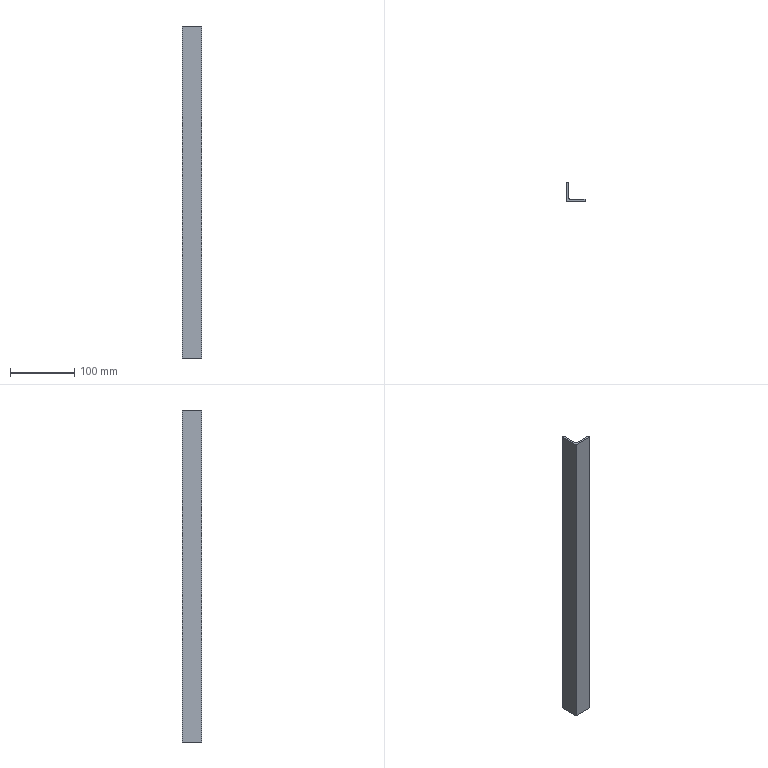Part | SolidWorks | features Extrusion 1 | 1 solid | 11 faces | box 30 x 30 x 515 mm | volume 90082 mm3 | plane 8 | cylinder 3 | commonest cylinder face diameters 2 x2 9 x1
STEP:
#1=CARTESIAN_POINT('',(2.,30.,-257.5));
#2=VERTEX_POINT('',#1);
#3=CARTESIAN_POINT('',(3.,29.,-257.5));
#4=VERTEX_POINT('',#3);
#5=CARTESIAN_POINT('',(2.,29.,-257.5));
#6=DIRECTION('',(0.,0.,-1.));
#7=DIRECTION('',(-1.,0.,0.));
#8=AXIS2_PLACEMENT_3D('',#5,#6,#7);
#9=CIRCLE('',#8,1.);
#10=EDGE_CURVE('',#2,#4,#9,.T.);
#11=ORIENTED_EDGE('',*,*,#10,.F.);
#12=CARTESIAN_POINT('',(2.,30.,257.5));
#13=VERTEX_POINT('',#12);
#14=CARTESIAN_POINT('',(2.,30.,257.5));
#15=DIRECTION('',(0.,0.,-1.));
#16=VECTOR('',#15,1000.);
#17=LINE('',#14,#16);
#18=EDGE_CURVE('',#13,#2,#17,.T.);
#19=ORIENTED_EDGE('',*,*,#18,.F.);
#20=CARTESIAN_POINT('',(3.,29.,257.5));
#21=VERTEX_POINT('',#20);
#22=CARTESIAN_POINT('',(2.,29.,257.5));
#23=DIRECTION('',(0.,0.,-1.));
#24=DIRECTION('',(-1.,0.,0.));
#25=AXIS2_PLACEMENT_3D('',#22,#23,#24);
#26=CIRCLE('',#25,1.);
#27=EDGE_CURVE('',#13,#21,#26,.T.);
#28=ORIENTED_EDGE('',*,*,#27,.T.);
#29=CARTESIAN_POINT('',(3.,29.,257.5));
#30=DIRECTION('',(0.,0.,-1.));
#31=VECTOR('',#30,1000.);
#32=LINE('',#29,#31);
#33=EDGE_CURVE('',#21,#4,#32,.T.);
#34=ORIENTED_EDGE('',*,*,#33,.T.);
#35=EDGE_LOOP('',(#11,#19,#28,#34));
#36=FACE_OUTER_BOUND('',#35,.T.);
#37=CARTESIAN_POINT('',(2.,29.,257.5));
#38=DIRECTION('',(0.,0.,-1.));
#39=DIRECTION('',(-1.,0.,0.));
#40=AXIS2_PLACEMENT_3D('',#37,#38,#39);
#41=CYLINDRICAL_SURFACE('',#40,1.);
#42=ADVANCED_FACE('',(#36),#41,.T.);
#43=CARTESIAN_POINT('',(0.,30.,-257.5));
#44=VERTEX_POINT('',#43);
#45=CARTESIAN_POINT('',(0.,30.,-257.5));
#46=DIRECTION('',(1.,0.,0.));
#47=VECTOR('',#46,1000.);
#48=LINE('',#45,#47);
#49=EDGE_CURVE('',#44,#2,#48,.T.);
#50=ORIENTED_EDGE('',*,*,#49,.F.);
#51=CARTESIAN_POINT('',(0.,30.,257.5));
#52=VERTEX_POINT('',#51);
#53=CARTESIAN_POINT('',(0.,30.,257.5));
#54=DIRECTION('',(0.,0.,-1.));
#55=VECTOR('',#54,1000.);
#56=LINE('',#53,#55);
#57=EDGE_CURVE('',#52,#44,#56,.T.);
#58=ORIENTED_EDGE('',*,*,#57,.F.);
#59=CARTESIAN_POINT('',(0.,30.,257.5));
#60=DIRECTION('',(1.,0.,0.));
#61=VECTOR('',#60,1000.);
#62=LINE('',#59,#61);
#63=EDGE_CURVE('',#52,#13,#62,.T.);
#64=ORIENTED_EDGE('',*,*,#63,.T.);
#65=ORIENTED_EDGE('',*,*,#18,.T.);
#66=EDGE_LOOP('',(#50,#58,#64,#65));
#67=FACE_OUTER_BOUND('',#66,.T.);
#68=CARTESIAN_POINT('',(0.,30.,257.5));
#69=DIRECTION('',(0.,1.,0.));
#70=DIRECTION('',(0.,0.,1.));
#71=AXIS2_PLACEMENT_3D('',#68,#69,#70);
#72=PLANE('',#71);
#73=ADVANCED_FACE('',(#67),#72,.T.);
#74=CARTESIAN_POINT('',(0.,0.,-257.5));
#75=VERTEX_POINT('',#74);
#76=CARTESIAN_POINT('',(0.,0.,-257.5));
#77=DIRECTION('',(0.,1.,0.));
#78=VECTOR('',#77,1000.);
#79=LINE('',#76,#78);
#80=EDGE_CURVE('',#75,#44,#79,.T.);
#81=ORIENTED_EDGE('',*,*,#80,.F.);
#82=CARTESIAN_POINT('',(0.,0.,257.5));
#83=VERTEX_POINT('',#82);
#84=CARTESIAN_POINT('',(0.,0.,257.5));
#85=DIRECTION('',(0.,0.,-1.));
#86=VECTOR('',#85,1000.);
#87=LINE('',#84,#86);
#88=EDGE_CURVE('',#83,#75,#87,.T.);
#89=ORIENTED_EDGE('',*,*,#88,.F.);
#90=CARTESIAN_POINT('',(0.,0.,257.5));
#91=DIRECTION('',(0.,1.,0.));
#92=VECTOR('',#91,1000.);
#93=LINE('',#90,#92);
#94=EDGE_CURVE('',#83,#52,#93,.T.);
#95=ORIENTED_EDGE('',*,*,#94,.T.);
#96=ORIENTED_EDGE('',*,*,#57,.T.);
#97=EDGE_LOOP('',(#81,#89,#95,#96));
#98=FACE_OUTER_BOUND('',#97,.T.);
#99=CARTESIAN_POINT('',(0.,0.,257.5));
#100=DIRECTION('',(-1.,0.,0.));
#101=DIRECTION('',(0.,0.,1.));
#102=AXIS2_PLACEMENT_3D('',#99,#100,#101);
#103=PLANE('',#102);
#104=ADVANCED_FACE('',(#98),#103,.T.);
#105=CARTESIAN_POINT('',(30.,0.,-257.5));
#106=VERTEX_POINT('',#105);
#107=CARTESIAN_POINT('',(30.,0.,-257.5));
#108=DIRECTION('',(-1.,0.,0.));
#109=VECTOR('',#108,1000.);
#110=LINE('',#107,#109);
#111=EDGE_CURVE('',#106,#75,#110,.T.);
#112=ORIENTED_EDGE('',*,*,#111,.F.);
#113=CARTESIAN_POINT('',(30.,0.,257.5));
#114=VERTEX_POINT('',#113);
#115=CARTESIAN_POINT('',(30.,0.,257.5));
#116=DIRECTION('',(0.,0.,-1.));
#117=VECTOR('',#116,1000.);
#118=LINE('',#115,#117);
#119=EDGE_CURVE('',#114,#106,#118,.T.);
#120=ORIENTED_EDGE('',*,*,#119,.F.);
#121=CARTESIAN_POINT('',(30.,0.,257.5));
#122=DIRECTION('',(-1.,0.,0.));
#123=VECTOR('',#122,1000.);
#124=LINE('',#121,#123);
#125=EDGE_CURVE('',#114,#83,#124,.T.);
#126=ORIENTED_EDGE('',*,*,#125,.T.);
#127=ORIENTED_EDGE('',*,*,#88,.T.);
#128=EDGE_LOOP('',(#112,#120,#126,#127));
#129=FACE_OUTER_BOUND('',#128,.T.);
#130=CARTESIAN_POINT('',(30.,0.,257.5));
#131=DIRECTION('',(0.,-1.,0.));
#132=DIRECTION('',(0.,0.,-1.));
#133=AXIS2_PLACEMENT_3D('',#130,#131,#132);
#134=PLANE('',#133);
#135=ADVANCED_FACE('',(#129),#134,.T.);
#136=CARTESIAN_POINT('',(30.,2.,-257.5));
#137=VERTEX_POINT('',#136);
#138=CARTESIAN_POINT('',(30.,0.,-257.5));
#139=DIRECTION('',(0.,1.,0.));
#140=VECTOR('',#139,1000.);
#141=LINE('',#138,#140);
#142=EDGE_CURVE('',#106,#137,#141,.T.);
#143=ORIENTED_EDGE('',*,*,#142,.T.);
#144=CARTESIAN_POINT('',(30.,2.,257.5));
#145=VERTEX_POINT('',#144);
#146=CARTESIAN_POINT('',(30.,2.,257.5));
#147=DIRECTION('',(0.,0.,-1.));
#148=VECTOR('',#147,1000.);
#149=LINE('',#146,#148);
#150=EDGE_CURVE('',#145,#137,#149,.T.);
#151=ORIENTED_EDGE('',*,*,#150,.F.);
#152=CARTESIAN_POINT('',(30.,0.,257.5));
#153=DIRECTION('',(0.,1.,0.));
#154=VECTOR('',#153,1000.);
#155=LINE('',#152,#154);
#156=EDGE_CURVE('',#114,#145,#155,.T.);
#157=ORIENTED_EDGE('',*,*,#156,.F.);
#158=ORIENTED_EDGE('',*,*,#119,.T.);
#159=EDGE_LOOP('',(#143,#151,#157,#158));
#160=FACE_OUTER_BOUND('',#159,.T.);
#161=CARTESIAN_POINT('',(30.,0.,257.5));
#162=DIRECTION('',(-1.,0.,0.));
#163=DIRECTION('',(0.,0.,1.));
#164=AXIS2_PLACEMENT_3D('',#161,#162,#163);
#165=PLANE('',#164);
#166=ADVANCED_FACE('',(#160),#165,.F.);
#167=CARTESIAN_POINT('',(29.,3.,-257.5));
#168=VERTEX_POINT('',#167);
#169=CARTESIAN_POINT('',(29.,2.,-257.5));
#170=DIRECTION('',(0.,0.,1.));
#171=DIRECTION('',(1.,0.,0.));
#172=AXIS2_PLACEMENT_3D('',#169,#170,#171);
#173=CIRCLE('',#172,1.);
#174=EDGE_CURVE('',#137,#168,#173,.T.);
#175=ORIENTED_EDGE('',*,*,#174,.T.);
#176=CARTESIAN_POINT('',(29.,3.,257.5));
#177=VERTEX_POINT('',#176);
#178=CARTESIAN_POINT('',(29.,3.,257.5));
#179=DIRECTION('',(0.,0.,-1.));
#180=VECTOR('',#179,1000.);
#181=LINE('',#178,#180);
#182=EDGE_CURVE('',#177,#168,#181,.T.);
#183=ORIENTED_EDGE('',*,*,#182,.F.);
#184=CARTESIAN_POINT('',(29.,2.,257.5));
#185=DIRECTION('',(0.,0.,1.));
#186=DIRECTION('',(1.,0.,0.));
#187=AXIS2_PLACEMENT_3D('',#184,#185,#186);
#188=CIRCLE('',#187,1.);
#189=EDGE_CURVE('',#145,#177,#188,.T.);
#190=ORIENTED_EDGE('',*,*,#189,.F.);
#191=ORIENTED_EDGE('',*,*,#150,.T.);
#192=EDGE_LOOP('',(#175,#183,#190,#191));
#193=FACE_OUTER_BOUND('',#192,.T.);
#194=CARTESIAN_POINT('',(29.,2.,257.5));
#195=DIRECTION('',(0.,0.,-1.));
#196=DIRECTION('',(-1.,0.,0.));
#197=AXIS2_PLACEMENT_3D('',#194,#195,#196);
#198=CYLINDRICAL_SURFACE('',#197,1.);
#199=ADVANCED_FACE('',(#193),#198,.T.);
#200=CARTESIAN_POINT('',(7.5,3.,-257.5));
#201=VERTEX_POINT('',#200);
#202=CARTESIAN_POINT('',(7.5,3.,-257.5));
#203=DIRECTION('',(1.,0.,0.));
#204=VECTOR('',#203,1000.);
#205=LINE('',#202,#204);
#206=EDGE_CURVE('',#201,#168,#205,.T.);
#207=ORIENTED_EDGE('',*,*,#206,.F.);
#208=CARTESIAN_POINT('',(7.5,3.,257.5));
#209=VERTEX_POINT('',#208);
#210=CARTESIAN_POINT('',(7.5,3.,257.5));
#211=DIRECTION('',(0.,0.,-1.));
#212=VECTOR('',#211,1000.);
#213=LINE('',#210,#212);
#214=EDGE_CURVE('',#209,#201,#213,.T.);
#215=ORIENTED_EDGE('',*,*,#214,.F.);
#216=CARTESIAN_POINT('',(7.5,3.,257.5));
#217=DIRECTION('',(1.,0.,0.));
#218=VECTOR('',#217,1000.);
#219=LINE('',#216,#218);
#220=EDGE_CURVE('',#209,#177,#219,.T.);
#221=ORIENTED_EDGE('',*,*,#220,.T.);
#222=ORIENTED_EDGE('',*,*,#182,.T.);
#223=EDGE_LOOP('',(#207,#215,#221,#222));
#224=FACE_OUTER_BOUND('',#223,.T.);
#225=CARTESIAN_POINT('',(7.5,3.,257.5));
#226=DIRECTION('',(0.,1.,0.));
#227=DIRECTION('',(-1.,0.,0.));
#228=AXIS2_PLACEMENT_3D('',#225,#226,#227);
#229=PLANE('',#228);
#230=ADVANCED_FACE('',(#224),#229,.T.);
#231=CARTESIAN_POINT('',(3.,7.5,-257.5));
#232=VERTEX_POINT('',#231);
#233=CARTESIAN_POINT('',(7.5,7.5,-257.5));
#234=DIRECTION('',(0.,0.,-1.));
#235=DIRECTION('',(-1.,0.,0.));
#236=AXIS2_PLACEMENT_3D('',#233,#234,#235);
#237=CIRCLE('',#236,4.5);
#238=EDGE_CURVE('',#201,#232,#237,.T.);
#239=ORIENTED_EDGE('',*,*,#238,.T.);
#240=CARTESIAN_POINT('',(3.,7.5,257.5));
#241=VERTEX_POINT('',#240);
#242=CARTESIAN_POINT('',(3.,7.5,257.5));
#243=DIRECTION('',(0.,0.,-1.));
#244=VECTOR('',#243,1000.);
#245=LINE('',#242,#244);
#246=EDGE_CURVE('',#241,#232,#245,.T.);
#247=ORIENTED_EDGE('',*,*,#246,.F.);
#248=CARTESIAN_POINT('',(7.5,7.5,257.5));
#249=DIRECTION('',(0.,0.,-1.));
#250=DIRECTION('',(-1.,0.,0.));
#251=AXIS2_PLACEMENT_3D('',#248,#249,#250);
#252=CIRCLE('',#251,4.5);
#253=EDGE_CURVE('',#209,#241,#252,.T.);
#254=ORIENTED_EDGE('',*,*,#253,.F.);
#255=ORIENTED_EDGE('',*,*,#214,.T.);
#256=EDGE_LOOP('',(#239,#247,#254,#255));
#257=FACE_OUTER_BOUND('',#256,.T.);
#258=CARTESIAN_POINT('',(7.5,7.5,257.5));
#259=DIRECTION('',(0.,0.,-1.));
#260=DIRECTION('',(-1.,0.,0.));
#261=AXIS2_PLACEMENT_3D('',#258,#259,#260);
#262=CYLINDRICAL_SURFACE('',#261,4.5);
#263=ADVANCED_FACE('',(#257),#262,.F.);
#264=CARTESIAN_POINT('',(3.,29.,-257.5));
#265=DIRECTION('',(0.,-1.,0.));
#266=VECTOR('',#265,1000.);
#267=LINE('',#264,#266);
#268=EDGE_CURVE('',#4,#232,#267,.T.);
#269=ORIENTED_EDGE('',*,*,#268,.F.);
#270=ORIENTED_EDGE('',*,*,#33,.F.);
#271=CARTESIAN_POINT('',(3.,29.,257.5));
#272=DIRECTION('',(0.,-1.,0.));
#273=VECTOR('',#272,1000.);
#274=LINE('',#271,#273);
#275=EDGE_CURVE('',#21,#241,#274,.T.);
#276=ORIENTED_EDGE('',*,*,#275,.T.);
#277=ORIENTED_EDGE('',*,*,#246,.T.);
#278=EDGE_LOOP('',(#269,#270,#276,#277));
#279=FACE_OUTER_BOUND('',#278,.T.);
#280=CARTESIAN_POINT('',(3.,29.,257.5));
#281=DIRECTION('',(1.,0.,0.));
#282=DIRECTION('',(0.,1.,0.));
#283=AXIS2_PLACEMENT_3D('',#280,#281,#282);
#284=PLANE('',#283);
#285=ADVANCED_FACE('',(#279),#284,.T.);
#286=ORIENTED_EDGE('',*,*,#27,.F.);
#287=ORIENTED_EDGE('',*,*,#63,.F.);
#288=ORIENTED_EDGE('',*,*,#94,.F.);
#289=ORIENTED_EDGE('',*,*,#125,.F.);
#290=ORIENTED_EDGE('',*,*,#156,.T.);
#291=ORIENTED_EDGE('',*,*,#189,.T.);
#292=ORIENTED_EDGE('',*,*,#220,.F.);
#293=ORIENTED_EDGE('',*,*,#253,.T.);
#294=ORIENTED_EDGE('',*,*,#275,.F.);
#295=EDGE_LOOP('',(#286,#287,#288,#289,#290,#291,#292,#293,#294));
#296=FACE_OUTER_BOUND('',#295,.T.);
#297=CARTESIAN_POINT('',(2.,29.,257.5));
#298=DIRECTION('',(0.,0.,-1.));
#299=DIRECTION('',(-1.,0.,0.));
#300=AXIS2_PLACEMENT_3D('',#297,#298,#299);
#301=PLANE('',#300);
#302=ADVANCED_FACE('',(#296),#301,.F.);
#303=ORIENTED_EDGE('',*,*,#10,.T.);
#304=ORIENTED_EDGE('',*,*,#268,.T.);
#305=ORIENTED_EDGE('',*,*,#238,.F.);
#306=ORIENTED_EDGE('',*,*,#206,.T.);
#307=ORIENTED_EDGE('',*,*,#174,.F.);
#308=ORIENTED_EDGE('',*,*,#142,.F.);
#309=ORIENTED_EDGE('',*,*,#111,.T.);
#310=ORIENTED_EDGE('',*,*,#80,.T.);
#311=ORIENTED_EDGE('',*,*,#49,.T.);
#312=EDGE_LOOP('',(#303,#304,#305,#306,#307,#308,#309,#310,#311));
#313=FACE_OUTER_BOUND('',#312,.T.);
#314=CARTESIAN_POINT('',(2.,29.,-257.5));
#315=DIRECTION('',(0.,0.,-1.));
#316=DIRECTION('',(-1.,0.,0.));
#317=AXIS2_PLACEMENT_3D('',#314,#315,#316);
#318=PLANE('',#317);
#319=ADVANCED_FACE('',(#313),#318,.T.);
#320=CLOSED_SHELL('',(#42,#73,#104,#135,#166,#199,#230,#263,#285,#302,#319));
#321=MANIFOLD_SOLID_BREP('',#320);
#322=CARTESIAN_POINT('',(0.,0.,0.));
#323=DIRECTION('',(0.,0.,1.));
#324=DIRECTION('',(1.,0.,0.));
#325=AXIS2_PLACEMENT_3D('',#322,#323,#324);
#326=(LENGTH_UNIT()NAMED_UNIT(*)SI_UNIT(.MILLI.,.METRE.));
#327=UNCERTAINTY_MEASURE_WITH_UNIT(LENGTH_MEASURE(0.00001),#326,'','');
#328=(NAMED_UNIT(*)PLANE_ANGLE_UNIT()SI_UNIT($,.RADIAN.));
#329=(NAMED_UNIT(*)SI_UNIT($,.STERADIAN.)SOLID_ANGLE_UNIT());
#330=(GEOMETRIC_REPRESENTATION_CONTEXT(3)GLOBAL_UNCERTAINTY_ASSIGNED_CONTEXT((#327))GLOBAL_UNIT_ASSIGNED_CONTEXT((#326,#328,#329))REPRESENTATION_CONTEXT('',''));
#331=ADVANCED_BREP_SHAPE_REPRESENTATION('',(#321,#325),#330);